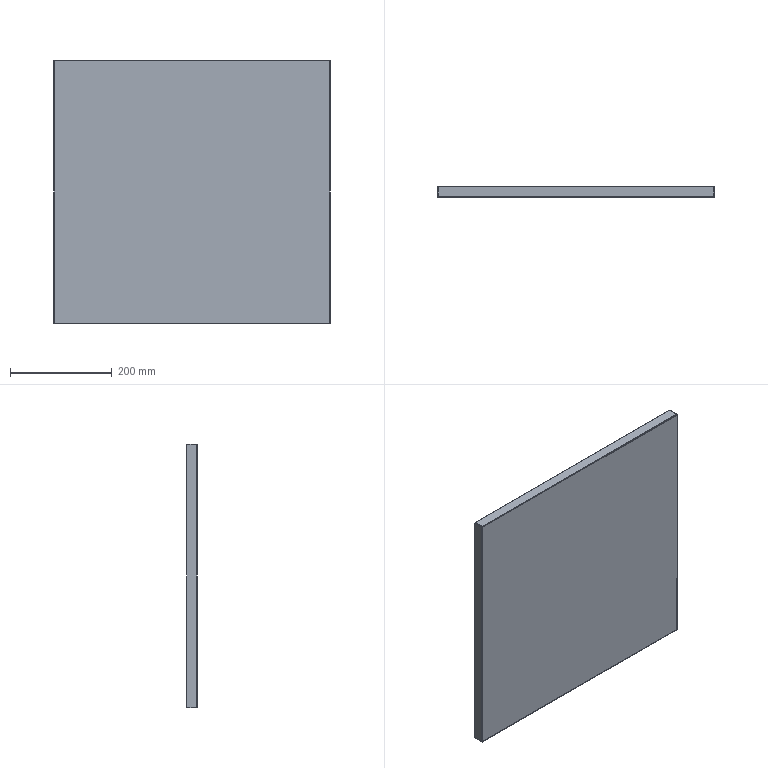Part | SolidWorks | features EdgeFlange 4, Cut 1, FlatPattern 1, SMBaseFlange 1, SheetMetal 1 | 1 solid | 38 faces | box 545 x 21 x 520 mm | volume 324842 mm3 | plane 30 | cylinder 8 | commonest cylinder face diameters 1 x4 3 x4
STEP:
#1=CARTESIAN_POINT('',(-271.,1.,-258.5));
#2=VERTEX_POINT('',#1);
#3=CARTESIAN_POINT('',(-271.,1.,258.5));
#4=VERTEX_POINT('',#3);
#5=CARTESIAN_POINT('',(-271.,1.,-258.5));
#6=DIRECTION('',(0.,0.,1.));
#7=VECTOR('',#6,1000.);
#8=LINE('',#5,#7);
#9=EDGE_CURVE('',#2,#4,#8,.T.);
#10=ORIENTED_EDGE('',*,*,#9,.T.);
#11=CARTESIAN_POINT('',(271.,1.,258.5));
#12=VERTEX_POINT('',#11);
#13=CARTESIAN_POINT('',(-271.,1.,258.5));
#14=DIRECTION('',(1.,0.,0.));
#15=VECTOR('',#14,1000.);
#16=LINE('',#13,#15);
#17=EDGE_CURVE('',#4,#12,#16,.T.);
#18=ORIENTED_EDGE('',*,*,#17,.T.);
#19=CARTESIAN_POINT('',(271.,1.,-258.5));
#20=VERTEX_POINT('',#19);
#21=CARTESIAN_POINT('',(271.,1.,-258.5));
#22=DIRECTION('',(0.,0.,-1.));
#23=VECTOR('',#22,1000.);
#24=LINE('',#21,#23);
#25=EDGE_CURVE('',#12,#20,#24,.T.);
#26=ORIENTED_EDGE('',*,*,#25,.T.);
#27=CARTESIAN_POINT('',(-271.,1.,-258.5));
#28=DIRECTION('',(-1.,0.,0.));
#29=VECTOR('',#28,1000.);
#30=LINE('',#27,#29);
#31=EDGE_CURVE('',#20,#2,#30,.T.);
#32=ORIENTED_EDGE('',*,*,#31,.T.);
#33=EDGE_LOOP('',(#10,#18,#26,#32));
#34=FACE_OUTER_BOUND('',#33,.T.);
#35=CARTESIAN_POINT('',(-271.,1.,258.5));
#36=DIRECTION('',(0.,1.,0.));
#37=DIRECTION('',(0.,0.,1.));
#38=AXIS2_PLACEMENT_3D('',#35,#36,#37);
#39=PLANE('',#38);
#40=ADVANCED_FACE('',(#34),#39,.T.);
#41=CARTESIAN_POINT('',(-271.,0.,-258.5));
#42=VERTEX_POINT('',#41);
#43=CARTESIAN_POINT('',(-271.,0.,258.5));
#44=VERTEX_POINT('',#43);
#45=CARTESIAN_POINT('',(-271.,0.,-258.5));
#46=DIRECTION('',(0.,0.,1.));
#47=VECTOR('',#46,1000.);
#48=LINE('',#45,#47);
#49=EDGE_CURVE('',#42,#44,#48,.T.);
#50=ORIENTED_EDGE('',*,*,#49,.F.);
#51=CARTESIAN_POINT('',(271.,0.,-258.5));
#52=VERTEX_POINT('',#51);
#53=CARTESIAN_POINT('',(-271.,0.,-258.5));
#54=DIRECTION('',(-1.,0.,0.));
#55=VECTOR('',#54,1000.);
#56=LINE('',#53,#55);
#57=EDGE_CURVE('',#52,#42,#56,.T.);
#58=ORIENTED_EDGE('',*,*,#57,.F.);
#59=CARTESIAN_POINT('',(271.,0.,258.5));
#60=VERTEX_POINT('',#59);
#61=CARTESIAN_POINT('',(271.,0.,-258.5));
#62=DIRECTION('',(0.,0.,-1.));
#63=VECTOR('',#62,1000.);
#64=LINE('',#61,#63);
#65=EDGE_CURVE('',#60,#52,#64,.T.);
#66=ORIENTED_EDGE('',*,*,#65,.F.);
#67=CARTESIAN_POINT('',(-271.,0.,258.5));
#68=DIRECTION('',(1.,0.,0.));
#69=VECTOR('',#68,1000.);
#70=LINE('',#67,#69);
#71=EDGE_CURVE('',#44,#60,#70,.T.);
#72=ORIENTED_EDGE('',*,*,#71,.F.);
#73=EDGE_LOOP('',(#50,#58,#66,#72));
#74=FACE_OUTER_BOUND('',#73,.T.);
#75=CARTESIAN_POINT('',(-271.,0.,258.5));
#76=DIRECTION('',(0.,1.,0.));
#77=DIRECTION('',(0.,0.,1.));
#78=AXIS2_PLACEMENT_3D('',#75,#76,#77);
#79=PLANE('',#78);
#80=ADVANCED_FACE('',(#74),#79,.F.);
#81=CARTESIAN_POINT('',(-271.5,1.5,-258.5));
#82=VERTEX_POINT('',#81);
#83=CARTESIAN_POINT('',(-272.5,1.5,-258.5));
#84=VERTEX_POINT('',#83);
#85=CARTESIAN_POINT('',(-272.5,1.5,-258.5));
#86=DIRECTION('',(-1.,0.,0.));
#87=VECTOR('',#86,1000.);
#88=LINE('',#85,#87);
#89=EDGE_CURVE('',#82,#84,#88,.T.);
#90=ORIENTED_EDGE('',*,*,#89,.F.);
#91=CARTESIAN_POINT('',(-271.,1.5,-258.5));
#92=DIRECTION('',(0.,0.,-1.));
#93=DIRECTION('',(1.,0.,0.));
#94=AXIS2_PLACEMENT_3D('',#91,#92,#93);
#95=CIRCLE('',#94,0.5);
#96=EDGE_CURVE('',#2,#82,#95,.T.);
#97=ORIENTED_EDGE('',*,*,#96,.F.);
#98=CARTESIAN_POINT('',(-271.,1.,-258.5));
#99=DIRECTION('',(0.,-1.,0.));
#100=VECTOR('',#99,1000.);
#101=LINE('',#98,#100);
#102=EDGE_CURVE('',#2,#42,#101,.T.);
#103=ORIENTED_EDGE('',*,*,#102,.T.);
#104=CARTESIAN_POINT('',(-271.,1.5,-258.5));
#105=DIRECTION('',(0.,0.,-1.));
#106=DIRECTION('',(1.,0.,0.));
#107=AXIS2_PLACEMENT_3D('',#104,#105,#106);
#108=CIRCLE('',#107,1.5);
#109=EDGE_CURVE('',#42,#84,#108,.T.);
#110=ORIENTED_EDGE('',*,*,#109,.T.);
#111=EDGE_LOOP('',(#90,#97,#103,#110));
#112=FACE_OUTER_BOUND('',#111,.T.);
#113=CARTESIAN_POINT('',(-271.,1.5,-258.5));
#114=DIRECTION('',(0.,0.,-1.));
#115=DIRECTION('',(-1.,0.,0.));
#116=AXIS2_PLACEMENT_3D('',#113,#114,#115);
#117=PLANE('',#116);
#118=ADVANCED_FACE('',(#112),#117,.T.);
#119=ORIENTED_EDGE('',*,*,#49,.T.);
#120=CARTESIAN_POINT('',(-272.5,1.5,258.5));
#121=VERTEX_POINT('',#120);
#122=CARTESIAN_POINT('',(-271.,1.5,258.5));
#123=DIRECTION('',(0.,0.,1.));
#124=DIRECTION('',(1.,0.,0.));
#125=AXIS2_PLACEMENT_3D('',#122,#123,#124);
#126=CIRCLE('',#125,1.5);
#127=EDGE_CURVE('',#121,#44,#126,.T.);
#128=ORIENTED_EDGE('',*,*,#127,.F.);
#129=CARTESIAN_POINT('',(-272.5,1.5,258.5));
#130=DIRECTION('',(0.,0.,1.));
#131=VECTOR('',#130,1000.);
#132=LINE('',#129,#131);
#133=EDGE_CURVE('',#84,#121,#132,.T.);
#134=ORIENTED_EDGE('',*,*,#133,.F.);
#135=ORIENTED_EDGE('',*,*,#109,.F.);
#136=EDGE_LOOP('',(#119,#128,#134,#135));
#137=FACE_OUTER_BOUND('',#136,.T.);
#138=CARTESIAN_POINT('',(-271.,1.5,258.5));
#139=DIRECTION('',(0.,0.,1.));
#140=DIRECTION('',(-1.,0.,0.));
#141=AXIS2_PLACEMENT_3D('',#138,#139,#140);
#142=CYLINDRICAL_SURFACE('',#141,1.5);
#143=ADVANCED_FACE('',(#137),#142,.T.);
#144=CARTESIAN_POINT('',(-271.5,1.5,258.5));
#145=VERTEX_POINT('',#144);
#146=CARTESIAN_POINT('',(-271.,1.5,258.5));
#147=DIRECTION('',(0.,0.,1.));
#148=DIRECTION('',(1.,0.,0.));
#149=AXIS2_PLACEMENT_3D('',#146,#147,#148);
#150=CIRCLE('',#149,0.5);
#151=EDGE_CURVE('',#145,#4,#150,.T.);
#152=ORIENTED_EDGE('',*,*,#151,.F.);
#153=CARTESIAN_POINT('',(-271.5,1.5,258.5));
#154=DIRECTION('',(-1.,0.,0.));
#155=VECTOR('',#154,1000.);
#156=LINE('',#153,#155);
#157=EDGE_CURVE('',#145,#121,#156,.T.);
#158=ORIENTED_EDGE('',*,*,#157,.T.);
#159=ORIENTED_EDGE('',*,*,#127,.T.);
#160=CARTESIAN_POINT('',(-271.,1.,258.5));
#161=DIRECTION('',(0.,-1.,0.));
#162=VECTOR('',#161,1000.);
#163=LINE('',#160,#162);
#164=EDGE_CURVE('',#4,#44,#163,.T.);
#165=ORIENTED_EDGE('',*,*,#164,.F.);
#166=EDGE_LOOP('',(#152,#158,#159,#165));
#167=FACE_OUTER_BOUND('',#166,.T.);
#168=CARTESIAN_POINT('',(-271.,1.5,258.5));
#169=DIRECTION('',(0.,0.,-1.));
#170=DIRECTION('',(-1.,0.,0.));
#171=AXIS2_PLACEMENT_3D('',#168,#169,#170);
#172=PLANE('',#171);
#173=ADVANCED_FACE('',(#167),#172,.F.);
#174=ORIENTED_EDGE('',*,*,#9,.F.);
#175=ORIENTED_EDGE('',*,*,#96,.T.);
#176=CARTESIAN_POINT('',(-271.5,1.5,-258.5));
#177=DIRECTION('',(0.,0.,1.));
#178=VECTOR('',#177,1000.);
#179=LINE('',#176,#178);
#180=EDGE_CURVE('',#82,#145,#179,.T.);
#181=ORIENTED_EDGE('',*,*,#180,.T.);
#182=ORIENTED_EDGE('',*,*,#151,.T.);
#183=EDGE_LOOP('',(#174,#175,#181,#182));
#184=FACE_OUTER_BOUND('',#183,.T.);
#185=CARTESIAN_POINT('',(-271.,1.5,258.5));
#186=DIRECTION('',(0.,0.,1.));
#187=DIRECTION('',(-1.,0.,0.));
#188=AXIS2_PLACEMENT_3D('',#185,#186,#187);
#189=CYLINDRICAL_SURFACE('',#188,0.5);
#190=ADVANCED_FACE('',(#184),#189,.F.);
#191=CARTESIAN_POINT('',(-272.5,21.,258.5));
#192=VERTEX_POINT('',#191);
#193=CARTESIAN_POINT('',(-272.5,1.,258.5));
#194=DIRECTION('',(0.,-1.,0.));
#195=VECTOR('',#194,1000.);
#196=LINE('',#193,#195);
#197=EDGE_CURVE('',#192,#121,#196,.T.);
#198=ORIENTED_EDGE('',*,*,#197,.T.);
#199=ORIENTED_EDGE('',*,*,#157,.F.);
#200=CARTESIAN_POINT('',(-271.5,21.,258.5));
#201=VERTEX_POINT('',#200);
#202=CARTESIAN_POINT('',(-271.5,1.,258.5));
#203=DIRECTION('',(0.,-1.,0.));
#204=VECTOR('',#203,1000.);
#205=LINE('',#202,#204);
#206=EDGE_CURVE('',#201,#145,#205,.T.);
#207=ORIENTED_EDGE('',*,*,#206,.F.);
#208=CARTESIAN_POINT('',(-272.5,21.,258.5));
#209=DIRECTION('',(1.,0.,0.));
#210=VECTOR('',#209,1000.);
#211=LINE('',#208,#210);
#212=EDGE_CURVE('',#192,#201,#211,.T.);
#213=ORIENTED_EDGE('',*,*,#212,.F.);
#214=EDGE_LOOP('',(#198,#199,#207,#213));
#215=FACE_OUTER_BOUND('',#214,.T.);
#216=CARTESIAN_POINT('',(-272.5,1.,258.5));
#217=DIRECTION('',(0.,0.,1.));
#218=DIRECTION('',(1.,0.,0.));
#219=AXIS2_PLACEMENT_3D('',#216,#217,#218);
#220=PLANE('',#219);
#221=ADVANCED_FACE('',(#215),#220,.T.);
#222=CARTESIAN_POINT('',(-271.5,21.,-258.5));
#223=VERTEX_POINT('',#222);
#224=CARTESIAN_POINT('',(-271.5,1.,-258.5));
#225=DIRECTION('',(0.,1.,0.));
#226=VECTOR('',#225,1000.);
#227=LINE('',#224,#226);
#228=EDGE_CURVE('',#82,#223,#227,.T.);
#229=ORIENTED_EDGE('',*,*,#228,.F.);
#230=ORIENTED_EDGE('',*,*,#89,.T.);
#231=CARTESIAN_POINT('',(-272.5,21.,-258.5));
#232=VERTEX_POINT('',#231);
#233=CARTESIAN_POINT('',(-272.5,21.,-258.5));
#234=DIRECTION('',(0.,1.,0.));
#235=VECTOR('',#234,1000.);
#236=LINE('',#233,#235);
#237=EDGE_CURVE('',#84,#232,#236,.T.);
#238=ORIENTED_EDGE('',*,*,#237,.T.);
#239=CARTESIAN_POINT('',(-272.5,21.,-258.5));
#240=DIRECTION('',(1.,0.,0.));
#241=VECTOR('',#240,1000.);
#242=LINE('',#239,#241);
#243=EDGE_CURVE('',#232,#223,#242,.T.);
#244=ORIENTED_EDGE('',*,*,#243,.T.);
#245=EDGE_LOOP('',(#229,#230,#238,#244));
#246=FACE_OUTER_BOUND('',#245,.T.);
#247=CARTESIAN_POINT('',(-272.5,21.,-258.5));
#248=DIRECTION('',(0.,0.,-1.));
#249=DIRECTION('',(0.,1.,0.));
#250=AXIS2_PLACEMENT_3D('',#247,#248,#249);
#251=PLANE('',#250);
#252=ADVANCED_FACE('',(#246),#251,.T.);
#253=ORIENTED_EDGE('',*,*,#237,.F.);
#254=ORIENTED_EDGE('',*,*,#133,.T.);
#255=ORIENTED_EDGE('',*,*,#197,.F.);
#256=CARTESIAN_POINT('',(-272.5,21.,258.5));
#257=DIRECTION('',(0.,0.,1.));
#258=VECTOR('',#257,1000.);
#259=LINE('',#256,#258);
#260=EDGE_CURVE('',#232,#192,#259,.T.);
#261=ORIENTED_EDGE('',*,*,#260,.F.);
#262=EDGE_LOOP('',(#253,#254,#255,#261));
#263=FACE_OUTER_BOUND('',#262,.T.);
#264=CARTESIAN_POINT('',(-272.5,1.,258.5));
#265=DIRECTION('',(-1.,0.,0.));
#266=DIRECTION('',(0.,-1.,0.));
#267=AXIS2_PLACEMENT_3D('',#264,#265,#266);
#268=PLANE('',#267);
#269=ADVANCED_FACE('',(#263),#268,.T.);
#270=ORIENTED_EDGE('',*,*,#180,.F.);
#271=ORIENTED_EDGE('',*,*,#228,.T.);
#272=CARTESIAN_POINT('',(-271.5,21.,258.5));
#273=DIRECTION('',(0.,0.,1.));
#274=VECTOR('',#273,1000.);
#275=LINE('',#272,#274);
#276=EDGE_CURVE('',#223,#201,#275,.T.);
#277=ORIENTED_EDGE('',*,*,#276,.T.);
#278=ORIENTED_EDGE('',*,*,#206,.T.);
#279=EDGE_LOOP('',(#270,#271,#277,#278));
#280=FACE_OUTER_BOUND('',#279,.T.);
#281=CARTESIAN_POINT('',(-271.5,1.,258.5));
#282=DIRECTION('',(-1.,0.,0.));
#283=DIRECTION('',(0.,-1.,0.));
#284=AXIS2_PLACEMENT_3D('',#281,#282,#283);
#285=PLANE('',#284);
#286=ADVANCED_FACE('',(#280),#285,.F.);
#287=ORIENTED_EDGE('',*,*,#276,.F.);
#288=ORIENTED_EDGE('',*,*,#243,.F.);
#289=ORIENTED_EDGE('',*,*,#260,.T.);
#290=ORIENTED_EDGE('',*,*,#212,.T.);
#291=EDGE_LOOP('',(#287,#288,#289,#290));
#292=FACE_OUTER_BOUND('',#291,.T.);
#293=CARTESIAN_POINT('',(-272.5,21.,258.5));
#294=DIRECTION('',(0.,1.,0.));
#295=DIRECTION('',(-1.,0.,0.));
#296=AXIS2_PLACEMENT_3D('',#293,#294,#295);
#297=PLANE('',#296);
#298=ADVANCED_FACE('',(#292),#297,.T.);
#299=CARTESIAN_POINT('',(271.5,1.5,258.5));
#300=VERTEX_POINT('',#299);
#301=CARTESIAN_POINT('',(272.5,1.5,258.5));
#302=VERTEX_POINT('',#301);
#303=CARTESIAN_POINT('',(272.5,1.5,258.5));
#304=DIRECTION('',(1.,0.,0.));
#305=VECTOR('',#304,1000.);
#306=LINE('',#303,#305);
#307=EDGE_CURVE('',#300,#302,#306,.T.);
#308=ORIENTED_EDGE('',*,*,#307,.F.);
#309=CARTESIAN_POINT('',(271.,1.5,258.5));
#310=DIRECTION('',(0.,0.,1.));
#311=DIRECTION('',(-1.,0.,0.));
#312=AXIS2_PLACEMENT_3D('',#309,#310,#311);
#313=CIRCLE('',#312,0.5);
#314=EDGE_CURVE('',#12,#300,#313,.T.);
#315=ORIENTED_EDGE('',*,*,#314,.F.);
#316=CARTESIAN_POINT('',(271.,1.,258.5));
#317=DIRECTION('',(0.,-1.,0.));
#318=VECTOR('',#317,1000.);
#319=LINE('',#316,#318);
#320=EDGE_CURVE('',#12,#60,#319,.T.);
#321=ORIENTED_EDGE('',*,*,#320,.T.);
#322=CARTESIAN_POINT('',(271.,1.5,258.5));
#323=DIRECTION('',(0.,0.,1.));
#324=DIRECTION('',(-1.,0.,0.));
#325=AXIS2_PLACEMENT_3D('',#322,#323,#324);
#326=CIRCLE('',#325,1.5);
#327=EDGE_CURVE('',#60,#302,#326,.T.);
#328=ORIENTED_EDGE('',*,*,#327,.T.);
#329=EDGE_LOOP('',(#308,#315,#321,#328));
#330=FACE_OUTER_BOUND('',#329,.T.);
#331=CARTESIAN_POINT('',(271.,1.5,258.5));
#332=DIRECTION('',(0.,0.,1.));
#333=DIRECTION('',(1.,0.,0.));
#334=AXIS2_PLACEMENT_3D('',#331,#332,#333);
#335=PLANE('',#334);
#336=ADVANCED_FACE('',(#330),#335,.T.);
#337=ORIENTED_EDGE('',*,*,#65,.T.);
#338=CARTESIAN_POINT('',(272.5,1.5,-258.5));
#339=VERTEX_POINT('',#338);
#340=CARTESIAN_POINT('',(271.,1.5,-258.5));
#341=DIRECTION('',(0.,0.,-1.));
#342=DIRECTION('',(-1.,0.,0.));
#343=AXIS2_PLACEMENT_3D('',#340,#341,#342);
#344=CIRCLE('',#343,1.5);
#345=EDGE_CURVE('',#339,#52,#344,.T.);
#346=ORIENTED_EDGE('',*,*,#345,.F.);
#347=CARTESIAN_POINT('',(272.5,1.5,-258.5));
#348=DIRECTION('',(0.,0.,-1.));
#349=VECTOR('',#348,1000.);
#350=LINE('',#347,#349);
#351=EDGE_CURVE('',#302,#339,#350,.T.);
#352=ORIENTED_EDGE('',*,*,#351,.F.);
#353=ORIENTED_EDGE('',*,*,#327,.F.);
#354=EDGE_LOOP('',(#337,#346,#352,#353));
#355=FACE_OUTER_BOUND('',#354,.T.);
#356=CARTESIAN_POINT('',(271.,1.5,-258.5));
#357=DIRECTION('',(0.,0.,-1.));
#358=DIRECTION('',(1.,0.,0.));
#359=AXIS2_PLACEMENT_3D('',#356,#357,#358);
#360=CYLINDRICAL_SURFACE('',#359,1.5);
#361=ADVANCED_FACE('',(#355),#360,.T.);
#362=CARTESIAN_POINT('',(271.5,1.5,-258.5));
#363=VERTEX_POINT('',#362);
#364=CARTESIAN_POINT('',(271.,1.5,-258.5));
#365=DIRECTION('',(0.,0.,-1.));
#366=DIRECTION('',(-1.,0.,0.));
#367=AXIS2_PLACEMENT_3D('',#364,#365,#366);
#368=CIRCLE('',#367,0.5);
#369=EDGE_CURVE('',#363,#20,#368,.T.);
#370=ORIENTED_EDGE('',*,*,#369,.F.);
#371=CARTESIAN_POINT('',(271.5,1.5,-258.5));
#372=DIRECTION('',(1.,0.,0.));
#373=VECTOR('',#372,1000.);
#374=LINE('',#371,#373);
#375=EDGE_CURVE('',#363,#339,#374,.T.);
#376=ORIENTED_EDGE('',*,*,#375,.T.);
#377=ORIENTED_EDGE('',*,*,#345,.T.);
#378=CARTESIAN_POINT('',(271.,1.,-258.5));
#379=DIRECTION('',(0.,-1.,0.));
#380=VECTOR('',#379,1000.);
#381=LINE('',#378,#380);
#382=EDGE_CURVE('',#20,#52,#381,.T.);
#383=ORIENTED_EDGE('',*,*,#382,.F.);
#384=EDGE_LOOP('',(#370,#376,#377,#383));
#385=FACE_OUTER_BOUND('',#384,.T.);
#386=CARTESIAN_POINT('',(271.,1.5,-258.5));
#387=DIRECTION('',(0.,0.,1.));
#388=DIRECTION('',(1.,0.,0.));
#389=AXIS2_PLACEMENT_3D('',#386,#387,#388);
#390=PLANE('',#389);
#391=ADVANCED_FACE('',(#385),#390,.F.);
#392=ORIENTED_EDGE('',*,*,#25,.F.);
#393=ORIENTED_EDGE('',*,*,#314,.T.);
#394=CARTESIAN_POINT('',(271.5,1.5,258.5));
#395=DIRECTION('',(0.,0.,-1.));
#396=VECTOR('',#395,1000.);
#397=LINE('',#394,#396);
#398=EDGE_CURVE('',#300,#363,#397,.T.);
#399=ORIENTED_EDGE('',*,*,#398,.T.);
#400=ORIENTED_EDGE('',*,*,#369,.T.);
#401=EDGE_LOOP('',(#392,#393,#399,#400));
#402=FACE_OUTER_BOUND('',#401,.T.);
#403=CARTESIAN_POINT('',(271.,1.5,-258.5));
#404=DIRECTION('',(0.,0.,-1.));
#405=DIRECTION('',(1.,0.,0.));
#406=AXIS2_PLACEMENT_3D('',#403,#404,#405);
#407=CYLINDRICAL_SURFACE('',#406,0.5);
#408=ADVANCED_FACE('',(#402),#407,.F.);
#409=CARTESIAN_POINT('',(272.5,21.,-258.5));
#410=VERTEX_POINT('',#409);
#411=CARTESIAN_POINT('',(272.5,1.,-258.5));
#412=DIRECTION('',(0.,-1.,0.));
#413=VECTOR('',#412,1000.);
#414=LINE('',#411,#413);
#415=EDGE_CURVE('',#410,#339,#414,.T.);
#416=ORIENTED_EDGE('',*,*,#415,.T.);
#417=ORIENTED_EDGE('',*,*,#375,.F.);
#418=CARTESIAN_POINT('',(271.5,21.,-258.5));
#419=VERTEX_POINT('',#418);
#420=CARTESIAN_POINT('',(271.5,1.,-258.5));
#421=DIRECTION('',(0.,-1.,0.));
#422=VECTOR('',#421,1000.);
#423=LINE('',#420,#422);
#424=EDGE_CURVE('',#419,#363,#423,.T.);
#425=ORIENTED_EDGE('',*,*,#424,.F.);
#426=CARTESIAN_POINT('',(272.5,21.,-258.5));
#427=DIRECTION('',(-1.,0.,0.));
#428=VECTOR('',#427,1000.);
#429=LINE('',#426,#428);
#430=EDGE_CURVE('',#410,#419,#429,.T.);
#431=ORIENTED_EDGE('',*,*,#430,.F.);
#432=EDGE_LOOP('',(#416,#417,#425,#431));
#433=FACE_OUTER_BOUND('',#432,.T.);
#434=CARTESIAN_POINT('',(272.5,1.,-258.5));
#435=DIRECTION('',(0.,0.,-1.));
#436=DIRECTION('',(0.,1.,0.));
#437=AXIS2_PLACEMENT_3D('',#434,#435,#436);
#438=PLANE('',#437);
#439=ADVANCED_FACE('',(#433),#438,.T.);
#440=CARTESIAN_POINT('',(271.5,21.,258.5));
#441=VERTEX_POINT('',#440);
#442=CARTESIAN_POINT('',(271.5,1.,258.5));
#443=DIRECTION('',(0.,1.,0.));
#444=VECTOR('',#443,1000.);
#445=LINE('',#442,#444);
#446=EDGE_CURVE('',#300,#441,#445,.T.);
#447=ORIENTED_EDGE('',*,*,#446,.F.);
#448=ORIENTED_EDGE('',*,*,#307,.T.);
#449=CARTESIAN_POINT('',(272.5,21.,258.5));
#450=VERTEX_POINT('',#449);
#451=CARTESIAN_POINT('',(272.5,21.,258.5));
#452=DIRECTION('',(0.,1.,0.));
#453=VECTOR('',#452,1000.);
#454=LINE('',#451,#453);
#455=EDGE_CURVE('',#302,#450,#454,.T.);
#456=ORIENTED_EDGE('',*,*,#455,.T.);
#457=CARTESIAN_POINT('',(272.5,21.,258.5));
#458=DIRECTION('',(-1.,0.,0.));
#459=VECTOR('',#458,1000.);
#460=LINE('',#457,#459);
#461=EDGE_CURVE('',#450,#441,#460,.T.);
#462=ORIENTED_EDGE('',*,*,#461,.T.);
#463=EDGE_LOOP('',(#447,#448,#456,#462));
#464=FACE_OUTER_BOUND('',#463,.T.);
#465=CARTESIAN_POINT('',(272.5,21.,258.5));
#466=DIRECTION('',(0.,0.,1.));
#467=DIRECTION('',(0.,-1.,0.));
#468=AXIS2_PLACEMENT_3D('',#465,#466,#467);
#469=PLANE('',#468);
#470=ADVANCED_FACE('',(#464),#469,.T.);
#471=ORIENTED_EDGE('',*,*,#455,.F.);
#472=ORIENTED_EDGE('',*,*,#351,.T.);
#473=ORIENTED_EDGE('',*,*,#415,.F.);
#474=CARTESIAN_POINT('',(272.5,21.,-258.5));
#475=DIRECTION('',(0.,0.,-1.));
#476=VECTOR('',#475,1000.);
#477=LINE('',#474,#476);
#478=EDGE_CURVE('',#450,#410,#477,.T.);
#479=ORIENTED_EDGE('',*,*,#478,.F.);
#480=EDGE_LOOP('',(#471,#472,#473,#479));
#481=FACE_OUTER_BOUND('',#480,.T.);
#482=CARTESIAN_POINT('',(272.5,1.,-258.5));
#483=DIRECTION('',(1.,0.,0.));
#484=DIRECTION('',(0.,1.,0.));
#485=AXIS2_PLACEMENT_3D('',#482,#483,#484);
#486=PLANE('',#485);
#487=ADVANCED_FACE('',(#481),#486,.T.);
#488=ORIENTED_EDGE('',*,*,#398,.F.);
#489=ORIENTED_EDGE('',*,*,#446,.T.);
#490=CARTESIAN_POINT('',(271.5,21.,-258.5));
#491=DIRECTION('',(0.,0.,-1.));
#492=VECTOR('',#491,1000.);
#493=LINE('',#490,#492);
#494=EDGE_CURVE('',#441,#419,#493,.T.);
#495=ORIENTED_EDGE('',*,*,#494,.T.);
#496=ORIENTED_EDGE('',*,*,#424,.T.);
#497=EDGE_LOOP('',(#488,#489,#495,#496));
#498=FACE_OUTER_BOUND('',#497,.T.);
#499=CARTESIAN_POINT('',(271.5,1.,-258.5));
#500=DIRECTION('',(1.,0.,0.));
#501=DIRECTION('',(0.,1.,0.));
#502=AXIS2_PLACEMENT_3D('',#499,#500,#501);
#503=PLANE('',#502);
#504=ADVANCED_FACE('',(#498),#503,.F.);
#505=ORIENTED_EDGE('',*,*,#494,.F.);
#506=ORIENTED_EDGE('',*,*,#461,.F.);
#507=ORIENTED_EDGE('',*,*,#478,.T.);
#508=ORIENTED_EDGE('',*,*,#430,.T.);
#509=EDGE_LOOP('',(#505,#506,#507,#508));
#510=FACE_OUTER_BOUND('',#509,.T.);
#511=CARTESIAN_POINT('',(272.5,21.,-258.5));
#512=DIRECTION('',(0.,1.,0.));
#513=DIRECTION('',(-1.,0.,0.));
#514=AXIS2_PLACEMENT_3D('',#511,#512,#513);
#515=PLANE('',#514);
#516=ADVANCED_FACE('',(#510),#515,.T.);
#517=CARTESIAN_POINT('',(271.,1.5,-259.));
#518=VERTEX_POINT('',#517);
#519=CARTESIAN_POINT('',(271.,1.5,-260.));
#520=VERTEX_POINT('',#519);
#521=CARTESIAN_POINT('',(271.,1.5,-260.));
#522=DIRECTION('',(0.,0.,-1.));
#523=VECTOR('',#522,1000.);
#524=LINE('',#521,#523);
#525=EDGE_CURVE('',#518,#520,#524,.T.);
#526=ORIENTED_EDGE('',*,*,#525,.F.);
#527=CARTESIAN_POINT('',(271.,1.5,-258.5));
#528=DIRECTION('',(1.,0.,0.));
#529=DIRECTION('',(0.,0.,1.));
#530=AXIS2_PLACEMENT_3D('',#527,#528,#529);
#531=CIRCLE('',#530,0.5);
#532=EDGE_CURVE('',#20,#518,#531,.T.);
#533=ORIENTED_EDGE('',*,*,#532,.F.);
#534=ORIENTED_EDGE('',*,*,#382,.T.);
#535=CARTESIAN_POINT('',(271.,1.5,-258.5));
#536=DIRECTION('',(1.,0.,0.));
#537=DIRECTION('',(0.,0.,1.));
#538=AXIS2_PLACEMENT_3D('',#535,#536,#537);
#539=CIRCLE('',#538,1.5);
#540=EDGE_CURVE('',#52,#520,#539,.T.);
#541=ORIENTED_EDGE('',*,*,#540,.T.);
#542=EDGE_LOOP('',(#526,#533,#534,#541));
#543=FACE_OUTER_BOUND('',#542,.T.);
#544=CARTESIAN_POINT('',(271.,1.5,-258.5));
#545=DIRECTION('',(1.,0.,0.));
#546=DIRECTION('',(0.,0.,-1.));
#547=AXIS2_PLACEMENT_3D('',#544,#545,#546);
#548=PLANE('',#547);
#549=ADVANCED_FACE('',(#543),#548,.T.);
#550=ORIENTED_EDGE('',*,*,#57,.T.);
#551=CARTESIAN_POINT('',(-271.,1.5,-260.));
#552=VERTEX_POINT('',#551);
#553=CARTESIAN_POINT('',(-271.,1.5,-258.5));
#554=DIRECTION('',(-1.,0.,0.));
#555=DIRECTION('',(0.,0.,1.));
#556=AXIS2_PLACEMENT_3D('',#553,#554,#555);
#557=CIRCLE('',#556,1.5);
#558=EDGE_CURVE('',#552,#42,#557,.T.);
#559=ORIENTED_EDGE('',*,*,#558,.F.);
#560=CARTESIAN_POINT('',(-271.,1.5,-260.));
#561=DIRECTION('',(-1.,0.,0.));
#562=VECTOR('',#561,1000.);
#563=LINE('',#560,#562);
#564=EDGE_CURVE('',#520,#552,#563,.T.);
#565=ORIENTED_EDGE('',*,*,#564,.F.);
#566=ORIENTED_EDGE('',*,*,#540,.F.);
#567=EDGE_LOOP('',(#550,#559,#565,#566));
#568=FACE_OUTER_BOUND('',#567,.T.);
#569=CARTESIAN_POINT('',(-271.,1.5,-258.5));
#570=DIRECTION('',(-1.,0.,0.));
#571=DIRECTION('',(0.,0.,-1.));
#572=AXIS2_PLACEMENT_3D('',#569,#570,#571);
#573=CYLINDRICAL_SURFACE('',#572,1.5);
#574=ADVANCED_FACE('',(#568),#573,.T.);
#575=CARTESIAN_POINT('',(-271.,1.5,-259.));
#576=VERTEX_POINT('',#575);
#577=CARTESIAN_POINT('',(-271.,1.5,-258.5));
#578=DIRECTION('',(-1.,0.,0.));
#579=DIRECTION('',(0.,0.,1.));
#580=AXIS2_PLACEMENT_3D('',#577,#578,#579);
#581=CIRCLE('',#580,0.5);
#582=EDGE_CURVE('',#576,#2,#581,.T.);
#583=ORIENTED_EDGE('',*,*,#582,.F.);
#584=CARTESIAN_POINT('',(-271.,1.5,-259.));
#585=DIRECTION('',(0.,0.,-1.));
#586=VECTOR('',#585,1000.);
#587=LINE('',#584,#586);
#588=EDGE_CURVE('',#576,#552,#587,.T.);
#589=ORIENTED_EDGE('',*,*,#588,.T.);
#590=ORIENTED_EDGE('',*,*,#558,.T.);
#591=ORIENTED_EDGE('',*,*,#102,.F.);
#592=EDGE_LOOP('',(#583,#589,#590,#591));
#593=FACE_OUTER_BOUND('',#592,.T.);
#594=CARTESIAN_POINT('',(-271.,1.5,-258.5));
#595=DIRECTION('',(1.,0.,0.));
#596=DIRECTION('',(0.,0.,-1.));
#597=AXIS2_PLACEMENT_3D('',#594,#595,#596);
#598=PLANE('',#597);
#599=ADVANCED_FACE('',(#593),#598,.F.);
#600=ORIENTED_EDGE('',*,*,#31,.F.);
#601=ORIENTED_EDGE('',*,*,#532,.T.);
#602=CARTESIAN_POINT('',(271.,1.5,-259.));
#603=DIRECTION('',(-1.,0.,0.));
#604=VECTOR('',#603,1000.);
#605=LINE('',#602,#604);
#606=EDGE_CURVE('',#518,#576,#605,.T.);
#607=ORIENTED_EDGE('',*,*,#606,.T.);
#608=ORIENTED_EDGE('',*,*,#582,.T.);
#609=EDGE_LOOP('',(#600,#601,#607,#608));
#610=FACE_OUTER_BOUND('',#609,.T.);
#611=CARTESIAN_POINT('',(-271.,1.5,-258.5));
#612=DIRECTION('',(-1.,0.,0.));
#613=DIRECTION('',(0.,0.,-1.));
#614=AXIS2_PLACEMENT_3D('',#611,#612,#613);
#615=CYLINDRICAL_SURFACE('',#614,0.5);
#616=ADVANCED_FACE('',(#610),#615,.F.);
#617=CARTESIAN_POINT('',(-271.,21.,-260.));
#618=VERTEX_POINT('',#617);
#619=CARTESIAN_POINT('',(-271.,1.,-260.));
#620=DIRECTION('',(0.,-1.,0.));
#621=VECTOR('',#620,1000.);
#622=LINE('',#619,#621);
#623=EDGE_CURVE('',#618,#552,#622,.T.);
#624=ORIENTED_EDGE('',*,*,#623,.T.);
#625=ORIENTED_EDGE('',*,*,#588,.F.);
#626=CARTESIAN_POINT('',(-271.,21.,-259.));
#627=VERTEX_POINT('',#626);
#628=CARTESIAN_POINT('',(-271.,1.,-259.));
#629=DIRECTION('',(0.,-1.,0.));
#630=VECTOR('',#629,1000.);
#631=LINE('',#628,#630);
#632=EDGE_CURVE('',#627,#576,#631,.T.);
#633=ORIENTED_EDGE('',*,*,#632,.F.);
#634=CARTESIAN_POINT('',(-271.,21.,-260.));
#635=DIRECTION('',(0.,0.,1.));
#636=VECTOR('',#635,1000.);
#637=LINE('',#634,#636);
#638=EDGE_CURVE('',#618,#627,#637,.T.);
#639=ORIENTED_EDGE('',*,*,#638,.F.);
#640=EDGE_LOOP('',(#624,#625,#633,#639));
#641=FACE_OUTER_BOUND('',#640,.T.);
#642=CARTESIAN_POINT('',(-271.,1.,-260.));
#643=DIRECTION('',(-1.,0.,0.));
#644=DIRECTION('',(0.,0.,1.));
#645=AXIS2_PLACEMENT_3D('',#642,#643,#644);
#646=PLANE('',#645);
#647=ADVANCED_FACE('',(#641),#646,.T.);
#648=CARTESIAN_POINT('',(271.,21.,-259.));
#649=VERTEX_POINT('',#648);
#650=CARTESIAN_POINT('',(271.,1.,-259.));
#651=DIRECTION('',(0.,1.,0.));
#652=VECTOR('',#651,1000.);
#653=LINE('',#650,#652);
#654=EDGE_CURVE('',#518,#649,#653,.T.);
#655=ORIENTED_EDGE('',*,*,#654,.F.);
#656=ORIENTED_EDGE('',*,*,#525,.T.);
#657=CARTESIAN_POINT('',(271.,21.,-260.));
#658=VERTEX_POINT('',#657);
#659=CARTESIAN_POINT('',(271.,21.,-260.));
#660=DIRECTION('',(0.,1.,0.));
#661=VECTOR('',#660,1000.);
#662=LINE('',#659,#661);
#663=EDGE_CURVE('',#520,#658,#662,.T.);
#664=ORIENTED_EDGE('',*,*,#663,.T.);
#665=CARTESIAN_POINT('',(271.,21.,-260.));
#666=DIRECTION('',(0.,0.,1.));
#667=VECTOR('',#666,1000.);
#668=LINE('',#665,#667);
#669=EDGE_CURVE('',#658,#649,#668,.T.);
#670=ORIENTED_EDGE('',*,*,#669,.T.);
#671=EDGE_LOOP('',(#655,#656,#664,#670));
#672=FACE_OUTER_BOUND('',#671,.T.);
#673=CARTESIAN_POINT('',(271.,21.,-260.));
#674=DIRECTION('',(1.,0.,0.));
#675=DIRECTION('',(0.,0.,-1.));
#676=AXIS2_PLACEMENT_3D('',#673,#674,#675);
#677=PLANE('',#676);
#678=ADVANCED_FACE('',(#672),#677,.T.);
#679=ORIENTED_EDGE('',*,*,#663,.F.);
#680=ORIENTED_EDGE('',*,*,#564,.T.);
#681=ORIENTED_EDGE('',*,*,#623,.F.);
#682=CARTESIAN_POINT('',(-271.,21.,-260.));
#683=DIRECTION('',(-1.,0.,0.));
#684=VECTOR('',#683,1000.);
#685=LINE('',#682,#684);
#686=EDGE_CURVE('',#658,#618,#685,.T.);
#687=ORIENTED_EDGE('',*,*,#686,.F.);
#688=EDGE_LOOP('',(#679,#680,#681,#687));
#689=FACE_OUTER_BOUND('',#688,.T.);
#690=CARTESIAN_POINT('',(-271.,1.,-260.));
#691=DIRECTION('',(0.,0.,-1.));
#692=DIRECTION('',(-1.,0.,0.));
#693=AXIS2_PLACEMENT_3D('',#690,#691,#692);
#694=PLANE('',#693);
#695=ADVANCED_FACE('',(#689),#694,.T.);
#696=ORIENTED_EDGE('',*,*,#606,.F.);
#697=ORIENTED_EDGE('',*,*,#654,.T.);
#698=CARTESIAN_POINT('',(-271.,21.,-259.));
#699=DIRECTION('',(-1.,0.,0.));
#700=VECTOR('',#699,1000.);
#701=LINE('',#698,#700);
#702=EDGE_CURVE('',#649,#627,#701,.T.);
#703=ORIENTED_EDGE('',*,*,#702,.T.);
#704=ORIENTED_EDGE('',*,*,#632,.T.);
#705=EDGE_LOOP('',(#696,#697,#703,#704));
#706=FACE_OUTER_BOUND('',#705,.T.);
#707=CARTESIAN_POINT('',(-271.,1.,-259.));
#708=DIRECTION('',(0.,0.,-1.));
#709=DIRECTION('',(-1.,0.,0.));
#710=AXIS2_PLACEMENT_3D('',#707,#708,#709);
#711=PLANE('',#710);
#712=ADVANCED_FACE('',(#706),#711,.F.);
#713=ORIENTED_EDGE('',*,*,#702,.F.);
#714=ORIENTED_EDGE('',*,*,#669,.F.);
#715=ORIENTED_EDGE('',*,*,#686,.T.);
#716=ORIENTED_EDGE('',*,*,#638,.T.);
#717=EDGE_LOOP('',(#713,#714,#715,#716));
#718=FACE_OUTER_BOUND('',#717,.T.);
#719=CARTESIAN_POINT('',(-271.,21.,-260.));
#720=DIRECTION('',(0.,1.,0.));
#721=DIRECTION('',(0.,0.,1.));
#722=AXIS2_PLACEMENT_3D('',#719,#720,#721);
#723=PLANE('',#722);
#724=ADVANCED_FACE('',(#718),#723,.T.);
#725=CARTESIAN_POINT('',(-271.,1.5,259.));
#726=VERTEX_POINT('',#725);
#727=CARTESIAN_POINT('',(-271.,1.5,260.));
#728=VERTEX_POINT('',#727);
#729=CARTESIAN_POINT('',(-271.,1.5,260.));
#730=DIRECTION('',(0.,0.,1.));
#731=VECTOR('',#730,1000.);
#732=LINE('',#729,#731);
#733=EDGE_CURVE('',#726,#728,#732,.T.);
#734=ORIENTED_EDGE('',*,*,#733,.F.);
#735=CARTESIAN_POINT('',(-271.,1.5,258.5));
#736=DIRECTION('',(-1.,0.,0.));
#737=DIRECTION('',(0.,0.,-1.));
#738=AXIS2_PLACEMENT_3D('',#735,#736,#737);
#739=CIRCLE('',#738,0.5);
#740=EDGE_CURVE('',#4,#726,#739,.T.);
#741=ORIENTED_EDGE('',*,*,#740,.F.);
#742=ORIENTED_EDGE('',*,*,#164,.T.);
#743=CARTESIAN_POINT('',(-271.,1.5,258.5));
#744=DIRECTION('',(-1.,0.,0.));
#745=DIRECTION('',(0.,0.,-1.));
#746=AXIS2_PLACEMENT_3D('',#743,#744,#745);
#747=CIRCLE('',#746,1.5);
#748=EDGE_CURVE('',#44,#728,#747,.T.);
#749=ORIENTED_EDGE('',*,*,#748,.T.);
#750=EDGE_LOOP('',(#734,#741,#742,#749));
#751=FACE_OUTER_BOUND('',#750,.T.);
#752=CARTESIAN_POINT('',(-271.,1.5,258.5));
#753=DIRECTION('',(-1.,0.,0.));
#754=DIRECTION('',(0.,0.,1.));
#755=AXIS2_PLACEMENT_3D('',#752,#753,#754);
#756=PLANE('',#755);
#757=ADVANCED_FACE('',(#751),#756,.T.);
#758=ORIENTED_EDGE('',*,*,#71,.T.);
#759=CARTESIAN_POINT('',(271.,1.5,260.));
#760=VERTEX_POINT('',#759);
#761=CARTESIAN_POINT('',(271.,1.5,258.5));
#762=DIRECTION('',(1.,0.,0.));
#763=DIRECTION('',(0.,0.,-1.));
#764=AXIS2_PLACEMENT_3D('',#761,#762,#763);
#765=CIRCLE('',#764,1.5);
#766=EDGE_CURVE('',#760,#60,#765,.T.);
#767=ORIENTED_EDGE('',*,*,#766,.F.);
#768=CARTESIAN_POINT('',(271.,1.5,260.));
#769=DIRECTION('',(1.,0.,0.));
#770=VECTOR('',#769,1000.);
#771=LINE('',#768,#770);
#772=EDGE_CURVE('',#728,#760,#771,.T.);
#773=ORIENTED_EDGE('',*,*,#772,.F.);
#774=ORIENTED_EDGE('',*,*,#748,.F.);
#775=EDGE_LOOP('',(#758,#767,#773,#774));
#776=FACE_OUTER_BOUND('',#775,.T.);
#777=CARTESIAN_POINT('',(271.,1.5,258.5));
#778=DIRECTION('',(1.,0.,0.));
#779=DIRECTION('',(0.,0.,1.));
#780=AXIS2_PLACEMENT_3D('',#777,#778,#779);
#781=CYLINDRICAL_SURFACE('',#780,1.5);
#782=ADVANCED_FACE('',(#776),#781,.T.);
#783=CARTESIAN_POINT('',(271.,1.5,259.));
#784=VERTEX_POINT('',#783);
#785=CARTESIAN_POINT('',(271.,1.5,258.5));
#786=DIRECTION('',(1.,0.,0.));
#787=DIRECTION('',(0.,0.,-1.));
#788=AXIS2_PLACEMENT_3D('',#785,#786,#787);
#789=CIRCLE('',#788,0.5);
#790=EDGE_CURVE('',#784,#12,#789,.T.);
#791=ORIENTED_EDGE('',*,*,#790,.F.);
#792=CARTESIAN_POINT('',(271.,1.5,259.));
#793=DIRECTION('',(0.,0.,1.));
#794=VECTOR('',#793,1000.);
#795=LINE('',#792,#794);
#796=EDGE_CURVE('',#784,#760,#795,.T.);
#797=ORIENTED_EDGE('',*,*,#796,.T.);
#798=ORIENTED_EDGE('',*,*,#766,.T.);
#799=ORIENTED_EDGE('',*,*,#320,.F.);
#800=EDGE_LOOP('',(#791,#797,#798,#799));
#801=FACE_OUTER_BOUND('',#800,.T.);
#802=CARTESIAN_POINT('',(271.,1.5,258.5));
#803=DIRECTION('',(-1.,0.,0.));
#804=DIRECTION('',(0.,0.,1.));
#805=AXIS2_PLACEMENT_3D('',#802,#803,#804);
#806=PLANE('',#805);
#807=ADVANCED_FACE('',(#801),#806,.F.);
#808=ORIENTED_EDGE('',*,*,#17,.F.);
#809=ORIENTED_EDGE('',*,*,#740,.T.);
#810=CARTESIAN_POINT('',(-271.,1.5,259.));
#811=DIRECTION('',(1.,0.,0.));
#812=VECTOR('',#811,1000.);
#813=LINE('',#810,#812);
#814=EDGE_CURVE('',#726,#784,#813,.T.);
#815=ORIENTED_EDGE('',*,*,#814,.T.);
#816=ORIENTED_EDGE('',*,*,#790,.T.);
#817=EDGE_LOOP('',(#808,#809,#815,#816));
#818=FACE_OUTER_BOUND('',#817,.T.);
#819=CARTESIAN_POINT('',(271.,1.5,258.5));
#820=DIRECTION('',(1.,0.,0.));
#821=DIRECTION('',(0.,0.,1.));
#822=AXIS2_PLACEMENT_3D('',#819,#820,#821);
#823=CYLINDRICAL_SURFACE('',#822,0.5);
#824=ADVANCED_FACE('',(#818),#823,.F.);
#825=CARTESIAN_POINT('',(271.,21.,260.));
#826=VERTEX_POINT('',#825);
#827=CARTESIAN_POINT('',(271.,1.,260.));
#828=DIRECTION('',(0.,-1.,0.));
#829=VECTOR('',#828,1000.);
#830=LINE('',#827,#829);
#831=EDGE_CURVE('',#826,#760,#830,.T.);
#832=ORIENTED_EDGE('',*,*,#831,.T.);
#833=ORIENTED_EDGE('',*,*,#796,.F.);
#834=CARTESIAN_POINT('',(271.,21.,259.));
#835=VERTEX_POINT('',#834);
#836=CARTESIAN_POINT('',(271.,1.,259.));
#837=DIRECTION('',(0.,-1.,0.));
#838=VECTOR('',#837,1000.);
#839=LINE('',#836,#838);
#840=EDGE_CURVE('',#835,#784,#839,.T.);
#841=ORIENTED_EDGE('',*,*,#840,.F.);
#842=CARTESIAN_POINT('',(271.,21.,260.));
#843=DIRECTION('',(0.,0.,-1.));
#844=VECTOR('',#843,1000.);
#845=LINE('',#842,#844);
#846=EDGE_CURVE('',#826,#835,#845,.T.);
#847=ORIENTED_EDGE('',*,*,#846,.F.);
#848=EDGE_LOOP('',(#832,#833,#841,#847));
#849=FACE_OUTER_BOUND('',#848,.T.);
#850=CARTESIAN_POINT('',(271.,1.,260.));
#851=DIRECTION('',(1.,0.,0.));
#852=DIRECTION('',(0.,0.,-1.));
#853=AXIS2_PLACEMENT_3D('',#850,#851,#852);
#854=PLANE('',#853);
#855=ADVANCED_FACE('',(#849),#854,.T.);
#856=CARTESIAN_POINT('',(-271.,21.,259.));
#857=VERTEX_POINT('',#856);
#858=CARTESIAN_POINT('',(-271.,1.,259.));
#859=DIRECTION('',(0.,1.,0.));
#860=VECTOR('',#859,1000.);
#861=LINE('',#858,#860);
#862=EDGE_CURVE('',#726,#857,#861,.T.);
#863=ORIENTED_EDGE('',*,*,#862,.F.);
#864=ORIENTED_EDGE('',*,*,#733,.T.);
#865=CARTESIAN_POINT('',(-271.,21.,260.));
#866=VERTEX_POINT('',#865);
#867=CARTESIAN_POINT('',(-271.,21.,260.));
#868=DIRECTION('',(0.,1.,0.));
#869=VECTOR('',#868,1000.);
#870=LINE('',#867,#869);
#871=EDGE_CURVE('',#728,#866,#870,.T.);
#872=ORIENTED_EDGE('',*,*,#871,.T.);
#873=CARTESIAN_POINT('',(-271.,21.,260.));
#874=DIRECTION('',(0.,0.,-1.));
#875=VECTOR('',#874,1000.);
#876=LINE('',#873,#875);
#877=EDGE_CURVE('',#866,#857,#876,.T.);
#878=ORIENTED_EDGE('',*,*,#877,.T.);
#879=EDGE_LOOP('',(#863,#864,#872,#878));
#880=FACE_OUTER_BOUND('',#879,.T.);
#881=CARTESIAN_POINT('',(-271.,21.,260.));
#882=DIRECTION('',(-1.,0.,0.));
#883=DIRECTION('',(0.,0.,1.));
#884=AXIS2_PLACEMENT_3D('',#881,#882,#883);
#885=PLANE('',#884);
#886=ADVANCED_FACE('',(#880),#885,.T.);
#887=ORIENTED_EDGE('',*,*,#871,.F.);
#888=ORIENTED_EDGE('',*,*,#772,.T.);
#889=ORIENTED_EDGE('',*,*,#831,.F.);
#890=CARTESIAN_POINT('',(271.,21.,260.));
#891=DIRECTION('',(1.,0.,0.));
#892=VECTOR('',#891,1000.);
#893=LINE('',#890,#892);
#894=EDGE_CURVE('',#866,#826,#893,.T.);
#895=ORIENTED_EDGE('',*,*,#894,.F.);
#896=EDGE_LOOP('',(#887,#888,#889,#895));
#897=FACE_OUTER_BOUND('',#896,.T.);
#898=CARTESIAN_POINT('',(271.,1.,260.));
#899=DIRECTION('',(0.,0.,1.));
#900=DIRECTION('',(0.,-1.,0.));
#901=AXIS2_PLACEMENT_3D('',#898,#899,#900);
#902=PLANE('',#901);
#903=ADVANCED_FACE('',(#897),#902,.T.);
#904=ORIENTED_EDGE('',*,*,#814,.F.);
#905=ORIENTED_EDGE('',*,*,#862,.T.);
#906=CARTESIAN_POINT('',(271.,21.,259.));
#907=DIRECTION('',(1.,0.,0.));
#908=VECTOR('',#907,1000.);
#909=LINE('',#906,#908);
#910=EDGE_CURVE('',#857,#835,#909,.T.);
#911=ORIENTED_EDGE('',*,*,#910,.T.);
#912=ORIENTED_EDGE('',*,*,#840,.T.);
#913=EDGE_LOOP('',(#904,#905,#911,#912));
#914=FACE_OUTER_BOUND('',#913,.T.);
#915=CARTESIAN_POINT('',(271.,1.,259.));
#916=DIRECTION('',(0.,0.,1.));
#917=DIRECTION('',(0.,-1.,0.));
#918=AXIS2_PLACEMENT_3D('',#915,#916,#917);
#919=PLANE('',#918);
#920=ADVANCED_FACE('',(#914),#919,.F.);
#921=ORIENTED_EDGE('',*,*,#910,.F.);
#922=ORIENTED_EDGE('',*,*,#877,.F.);
#923=ORIENTED_EDGE('',*,*,#894,.T.);
#924=ORIENTED_EDGE('',*,*,#846,.T.);
#925=EDGE_LOOP('',(#921,#922,#923,#924));
#926=FACE_OUTER_BOUND('',#925,.T.);
#927=CARTESIAN_POINT('',(271.,21.,260.));
#928=DIRECTION('',(0.,1.,0.));
#929=DIRECTION('',(0.,0.,1.));
#930=AXIS2_PLACEMENT_3D('',#927,#928,#929);
#931=PLANE('',#930);
#932=ADVANCED_FACE('',(#926),#931,.T.);
#933=CLOSED_SHELL('',(#40,#80,#118,#143,#173,#190,#221,#252,#269,#286,#298,#336,#361,#391,#408,#439,#470,#487,#504,#516,#549,#574,#599,#616,#647,#678,#695,#712,#724,#757,#782,#807,#824,#855,#886,#903,#920,#932));
#934=MANIFOLD_SOLID_BREP('',#933);
#935=CARTESIAN_POINT('',(0.,0.,0.));
#936=DIRECTION('',(0.,0.,1.));
#937=DIRECTION('',(1.,0.,0.));
#938=AXIS2_PLACEMENT_3D('',#935,#936,#937);
#939=(LENGTH_UNIT()NAMED_UNIT(*)SI_UNIT(.MILLI.,.METRE.));
#940=UNCERTAINTY_MEASURE_WITH_UNIT(LENGTH_MEASURE(0.00001),#939,'','');
#941=(NAMED_UNIT(*)PLANE_ANGLE_UNIT()SI_UNIT($,.RADIAN.));
#942=(NAMED_UNIT(*)SI_UNIT($,.STERADIAN.)SOLID_ANGLE_UNIT());
#943=(GEOMETRIC_REPRESENTATION_CONTEXT(3)GLOBAL_UNCERTAINTY_ASSIGNED_CONTEXT((#940))GLOBAL_UNIT_ASSIGNED_CONTEXT((#939,#941,#942))REPRESENTATION_CONTEXT('',''));
#944=ADVANCED_BREP_SHAPE_REPRESENTATION('',(#934,#938),#943);